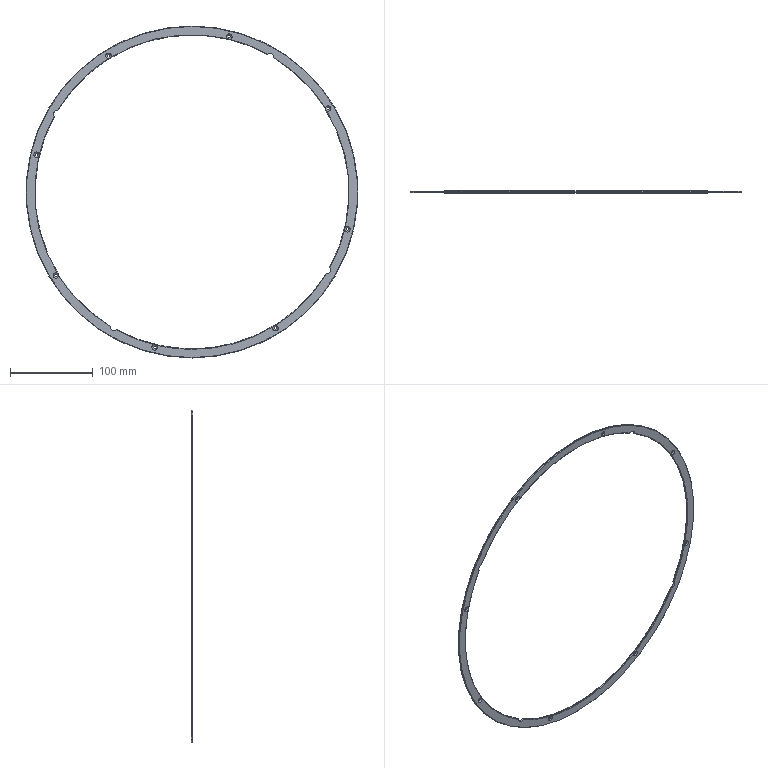Part | NX | features BREP 1 | 1 solid | 69 faces | box 402 x 2 x 402 mm | volume 25979 mm3 | cone 30 | cylinder 29 | plane 10 | commonest cylinder face diameters 3.4 x16 9 x6 380 x5 402 x2